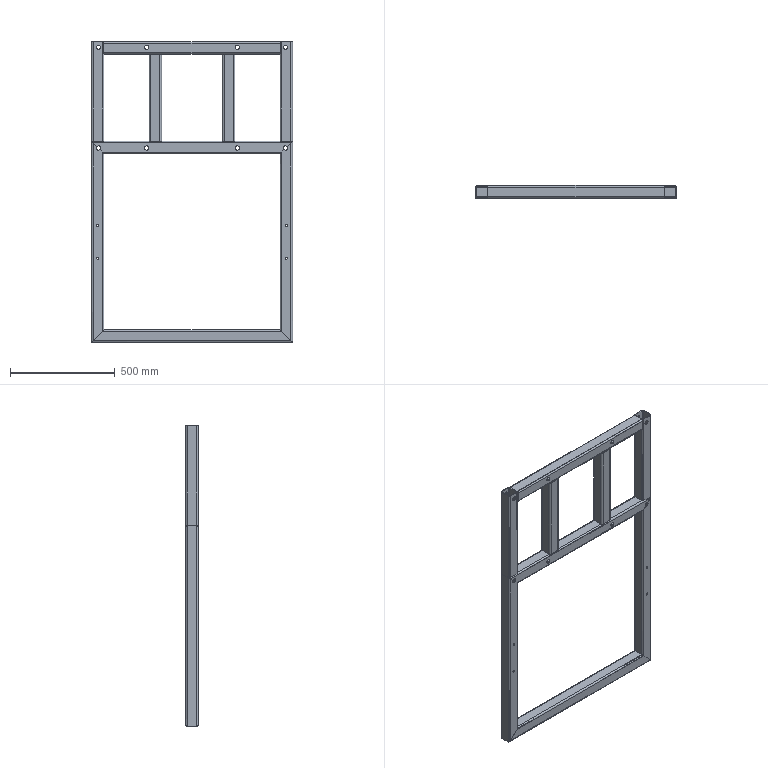Part | SolidWorks | features ICE 2, MirrorPattern 2, LPattern 1, WeldMemberFeat 1, WeldmentFeature 1 | 9 solids | 218 faces | box 960 x 60 x 1436 mm | volume 5295924 mm3 | cylinder 124 | plane 94 | commonest cylinder face diameters 8 x36 16 x36 20 x36 10 x16